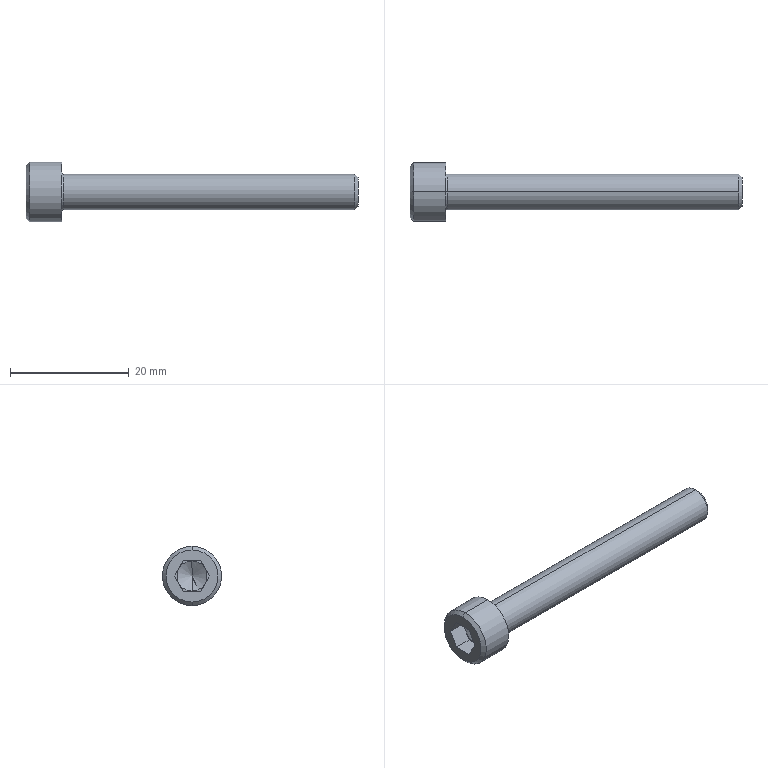Part | STEP file | socket head cap screw_am_B18.3.1M - 6 x 1.0 x 50 Hex SHCS -- 24NHX | 1 solid | 27 faces | box 56 x 10 x 10 mm | volume 1800 mm3 | plane 15 | cone 6 | cylinder 4 | torus 2 | commonest cylinder face diameters 6 x2 10 x2